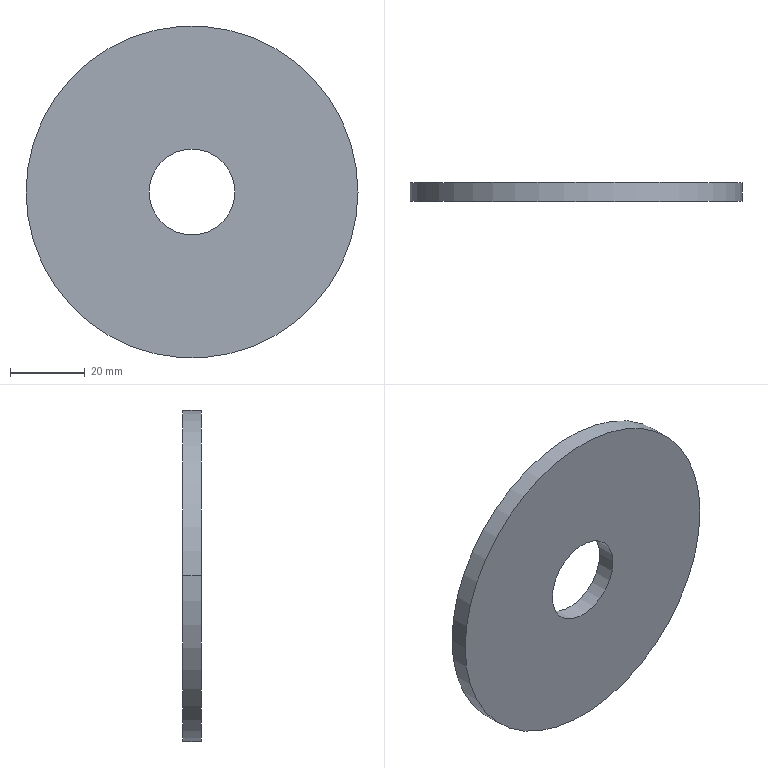Part | SolidWorks | features Revolution 1 | 1 solid | 6 faces | box 89 x 5 x 89 mm | volume 29028 mm3 | cylinder 4 | plane 2 | commonest cylinder face diameters 23 x2 89 x2
STEP:
#1=CARTESIAN_POINT('',(44.5,5.,0.));
#2=VERTEX_POINT('',#1);
#3=CARTESIAN_POINT('',(-44.5,5.,0.));
#4=VERTEX_POINT('',#3);
#5=CARTESIAN_POINT('',(0.,5.,0.));
#6=DIRECTION('',(0.,-1.,0.));
#7=DIRECTION('',(1.,0.,0.));
#8=AXIS2_PLACEMENT_3D('',#5,#6,#7);
#9=CIRCLE('',#8,44.5);
#10=EDGE_CURVE('',#2,#4,#9,.T.);
#11=ORIENTED_EDGE('',*,*,#10,.T.);
#12=CARTESIAN_POINT('',(-44.5,0.,0.));
#13=VERTEX_POINT('',#12);
#14=CARTESIAN_POINT('',(-44.5,-799.869,0.));
#15=DIRECTION('',(0.,-1.,0.));
#16=VECTOR('',#15,1000.);
#17=LINE('',#14,#16);
#18=EDGE_CURVE('',#4,#13,#17,.T.);
#19=ORIENTED_EDGE('',*,*,#18,.T.);
#20=CARTESIAN_POINT('',(44.5,0.,0.));
#21=VERTEX_POINT('',#20);
#22=CARTESIAN_POINT('',(0.,0.,0.));
#23=DIRECTION('',(0.,-1.,0.));
#24=DIRECTION('',(1.,0.,0.));
#25=AXIS2_PLACEMENT_3D('',#22,#23,#24);
#26=CIRCLE('',#25,44.5);
#27=EDGE_CURVE('',#21,#13,#26,.T.);
#28=ORIENTED_EDGE('',*,*,#27,.F.);
#29=CARTESIAN_POINT('',(44.5,-799.869,0.));
#30=DIRECTION('',(0.,-1.,0.));
#31=VECTOR('',#30,1000.);
#32=LINE('',#29,#31);
#33=EDGE_CURVE('',#2,#21,#32,.T.);
#34=ORIENTED_EDGE('',*,*,#33,.F.);
#35=EDGE_LOOP('',(#11,#19,#28,#34));
#36=FACE_OUTER_BOUND('',#35,.T.);
#37=CARTESIAN_POINT('',(0.,-799.869,0.));
#38=DIRECTION('',(0.,-1.,0.));
#39=DIRECTION('',(1.,0.,0.));
#40=AXIS2_PLACEMENT_3D('',#37,#38,#39);
#41=CYLINDRICAL_SURFACE('',#40,44.5);
#42=ADVANCED_FACE('',(#36),#41,.T.);
#43=CARTESIAN_POINT('',(-11.5,5.,0.));
#44=VERTEX_POINT('',#43);
#45=CARTESIAN_POINT('',(11.5,5.,0.));
#46=VERTEX_POINT('',#45);
#47=CARTESIAN_POINT('',(0.,5.,0.));
#48=DIRECTION('',(0.,-1.,0.));
#49=DIRECTION('',(1.,0.,0.));
#50=AXIS2_PLACEMENT_3D('',#47,#48,#49);
#51=CIRCLE('',#50,11.5);
#52=EDGE_CURVE('',#44,#46,#51,.T.);
#53=ORIENTED_EDGE('',*,*,#52,.F.);
#54=CARTESIAN_POINT('',(-11.5,0.,0.));
#55=VERTEX_POINT('',#54);
#56=CARTESIAN_POINT('',(-11.5,-799.869,0.));
#57=DIRECTION('',(0.,-1.,0.));
#58=VECTOR('',#57,1000.);
#59=LINE('',#56,#58);
#60=EDGE_CURVE('',#44,#55,#59,.T.);
#61=ORIENTED_EDGE('',*,*,#60,.T.);
#62=CARTESIAN_POINT('',(11.5,0.,0.));
#63=VERTEX_POINT('',#62);
#64=CARTESIAN_POINT('',(0.,0.,0.));
#65=DIRECTION('',(0.,-1.,0.));
#66=DIRECTION('',(1.,0.,0.));
#67=AXIS2_PLACEMENT_3D('',#64,#65,#66);
#68=CIRCLE('',#67,11.5);
#69=EDGE_CURVE('',#55,#63,#68,.T.);
#70=ORIENTED_EDGE('',*,*,#69,.T.);
#71=CARTESIAN_POINT('',(11.5,-799.869,0.));
#72=DIRECTION('',(0.,-1.,0.));
#73=VECTOR('',#72,1000.);
#74=LINE('',#71,#73);
#75=EDGE_CURVE('',#46,#63,#74,.T.);
#76=ORIENTED_EDGE('',*,*,#75,.F.);
#77=EDGE_LOOP('',(#53,#61,#70,#76));
#78=FACE_OUTER_BOUND('',#77,.T.);
#79=CARTESIAN_POINT('',(0.,-799.869,0.));
#80=DIRECTION('',(0.,-1.,0.));
#81=DIRECTION('',(1.,0.,0.));
#82=AXIS2_PLACEMENT_3D('',#79,#80,#81);
#83=CYLINDRICAL_SURFACE('',#82,11.5);
#84=ADVANCED_FACE('',(#78),#83,.F.);
#85=ORIENTED_EDGE('',*,*,#60,.F.);
#86=CARTESIAN_POINT('',(0.,5.,0.));
#87=DIRECTION('',(0.,-1.,0.));
#88=DIRECTION('',(1.,0.,0.));
#89=AXIS2_PLACEMENT_3D('',#86,#87,#88);
#90=CIRCLE('',#89,11.5);
#91=EDGE_CURVE('',#46,#44,#90,.T.);
#92=ORIENTED_EDGE('',*,*,#91,.F.);
#93=ORIENTED_EDGE('',*,*,#75,.T.);
#94=CARTESIAN_POINT('',(0.,0.,0.));
#95=DIRECTION('',(0.,-1.,0.));
#96=DIRECTION('',(1.,0.,0.));
#97=AXIS2_PLACEMENT_3D('',#94,#95,#96);
#98=CIRCLE('',#97,11.5);
#99=EDGE_CURVE('',#63,#55,#98,.T.);
#100=ORIENTED_EDGE('',*,*,#99,.T.);
#101=EDGE_LOOP('',(#85,#92,#93,#100));
#102=FACE_OUTER_BOUND('',#101,.T.);
#103=CARTESIAN_POINT('',(0.,-799.869,0.));
#104=DIRECTION('',(0.,-1.,0.));
#105=DIRECTION('',(1.,0.,0.));
#106=AXIS2_PLACEMENT_3D('',#103,#104,#105);
#107=CYLINDRICAL_SURFACE('',#106,11.5);
#108=ADVANCED_FACE('',(#102),#107,.F.);
#109=ORIENTED_EDGE('',*,*,#91,.T.);
#110=ORIENTED_EDGE('',*,*,#52,.T.);
#111=EDGE_LOOP('',(#109,#110));
#112=FACE_BOUND('',#111,.T.);
#113=ORIENTED_EDGE('',*,*,#10,.F.);
#114=CARTESIAN_POINT('',(0.,5.,0.));
#115=DIRECTION('',(0.,-1.,0.));
#116=DIRECTION('',(1.,0.,0.));
#117=AXIS2_PLACEMENT_3D('',#114,#115,#116);
#118=CIRCLE('',#117,44.5);
#119=EDGE_CURVE('',#4,#2,#118,.T.);
#120=ORIENTED_EDGE('',*,*,#119,.F.);
#121=EDGE_LOOP('',(#113,#120));
#122=FACE_OUTER_BOUND('',#121,.T.);
#123=CARTESIAN_POINT('',(11.5,5.,0.));
#124=DIRECTION('',(0.,1.,0.));
#125=DIRECTION('',(-1.,0.,0.));
#126=AXIS2_PLACEMENT_3D('',#123,#124,#125);
#127=PLANE('',#126);
#128=ADVANCED_FACE('',(#112,#122),#127,.T.);
#129=ORIENTED_EDGE('',*,*,#18,.F.);
#130=ORIENTED_EDGE('',*,*,#119,.T.);
#131=ORIENTED_EDGE('',*,*,#33,.T.);
#132=CARTESIAN_POINT('',(0.,0.,0.));
#133=DIRECTION('',(0.,-1.,0.));
#134=DIRECTION('',(1.,0.,0.));
#135=AXIS2_PLACEMENT_3D('',#132,#133,#134);
#136=CIRCLE('',#135,44.5);
#137=EDGE_CURVE('',#13,#21,#136,.T.);
#138=ORIENTED_EDGE('',*,*,#137,.F.);
#139=EDGE_LOOP('',(#129,#130,#131,#138));
#140=FACE_OUTER_BOUND('',#139,.T.);
#141=CARTESIAN_POINT('',(0.,-799.869,0.));
#142=DIRECTION('',(0.,-1.,0.));
#143=DIRECTION('',(1.,0.,0.));
#144=AXIS2_PLACEMENT_3D('',#141,#142,#143);
#145=CYLINDRICAL_SURFACE('',#144,44.5);
#146=ADVANCED_FACE('',(#140),#145,.T.);
#147=ORIENTED_EDGE('',*,*,#27,.T.);
#148=ORIENTED_EDGE('',*,*,#137,.T.);
#149=EDGE_LOOP('',(#147,#148));
#150=FACE_OUTER_BOUND('',#149,.T.);
#151=ORIENTED_EDGE('',*,*,#99,.F.);
#152=ORIENTED_EDGE('',*,*,#69,.F.);
#153=EDGE_LOOP('',(#151,#152));
#154=FACE_BOUND('',#153,.T.);
#155=CARTESIAN_POINT('',(11.5,0.,0.));
#156=DIRECTION('',(0.,-1.,0.));
#157=DIRECTION('',(1.,0.,0.));
#158=AXIS2_PLACEMENT_3D('',#155,#156,#157);
#159=PLANE('',#158);
#160=ADVANCED_FACE('',(#150,#154),#159,.T.);
#161=CLOSED_SHELL('',(#42,#84,#108,#128,#146,#160));
#162=MANIFOLD_SOLID_BREP('',#161);
#163=CARTESIAN_POINT('',(0.,0.,0.));
#164=DIRECTION('',(0.,0.,1.));
#165=DIRECTION('',(1.,0.,0.));
#166=AXIS2_PLACEMENT_3D('',#163,#164,#165);
#167=(LENGTH_UNIT()NAMED_UNIT(*)SI_UNIT(.MILLI.,.METRE.));
#168=UNCERTAINTY_MEASURE_WITH_UNIT(LENGTH_MEASURE(0.00001),#167,'','');
#169=(NAMED_UNIT(*)PLANE_ANGLE_UNIT()SI_UNIT($,.RADIAN.));
#170=(NAMED_UNIT(*)SI_UNIT($,.STERADIAN.)SOLID_ANGLE_UNIT());
#171=(GEOMETRIC_REPRESENTATION_CONTEXT(3)GLOBAL_UNCERTAINTY_ASSIGNED_CONTEXT((#168))GLOBAL_UNIT_ASSIGNED_CONTEXT((#167,#169,#170))REPRESENTATION_CONTEXT('',''));
#172=ADVANCED_BREP_SHAPE_REPRESENTATION('',(#162,#166),#171);